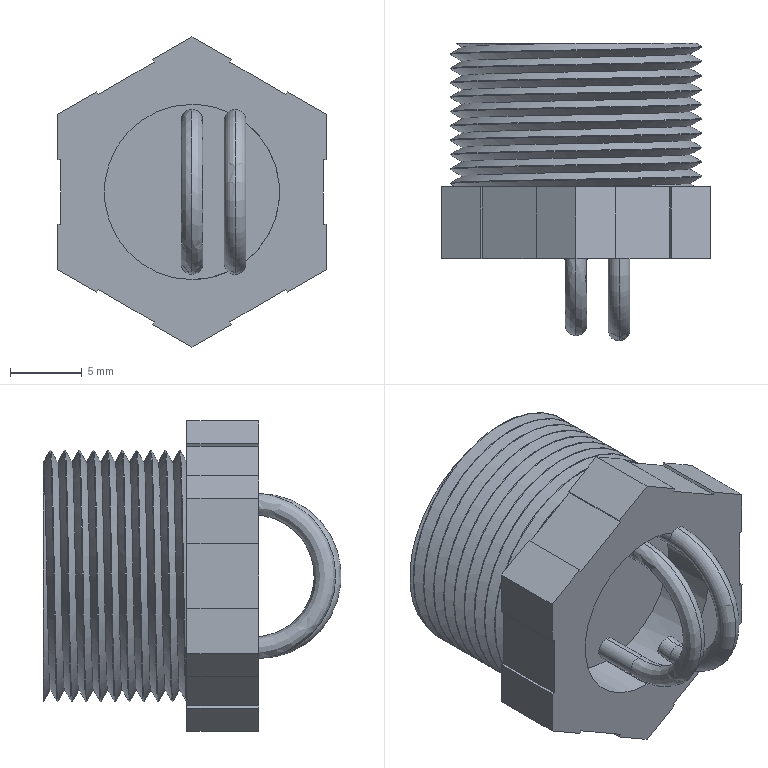Part | STEP file | 1 solid | 86 faces | box 18.7 x 20.75 x 21.593 mm | volume 2111 mm3 | cylinder 39 | plane 39 | torus 4 | spline 4 | commonest cylinder face diameters 17.5 x22 1.5 x12 12.2 x5